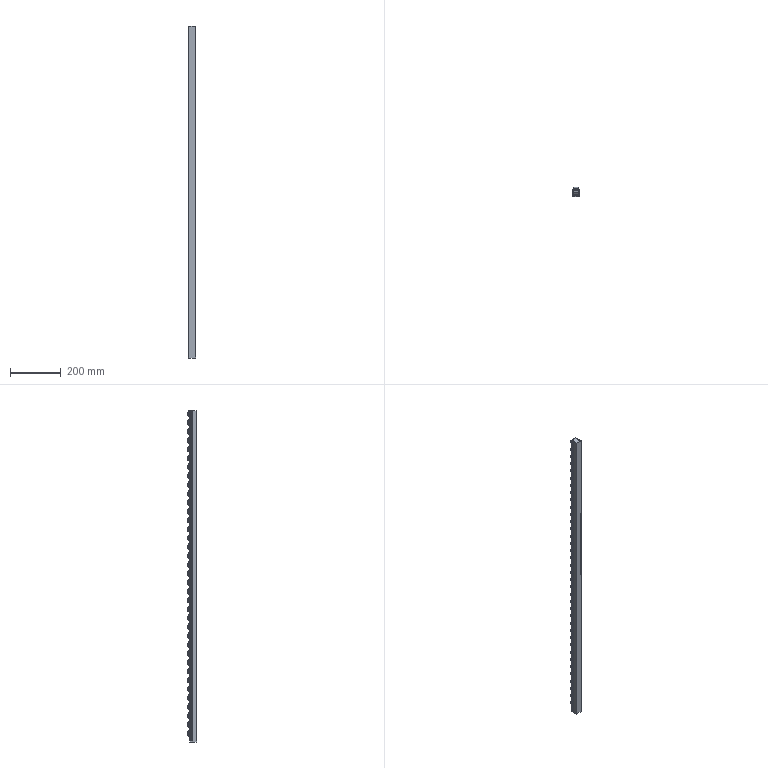Part | STEP file | RIEL FINAL NLV 2 | 47 solids | 1592 faces | box 28.4 x 36.2 x 1308 mm | volume 381210 mm3 | cylinder 814 | plane 706 | spline 72 | commonest cylinder face diameters 10 x296 25 x296 5 x74 30 x74 4 x58 1.473 x8